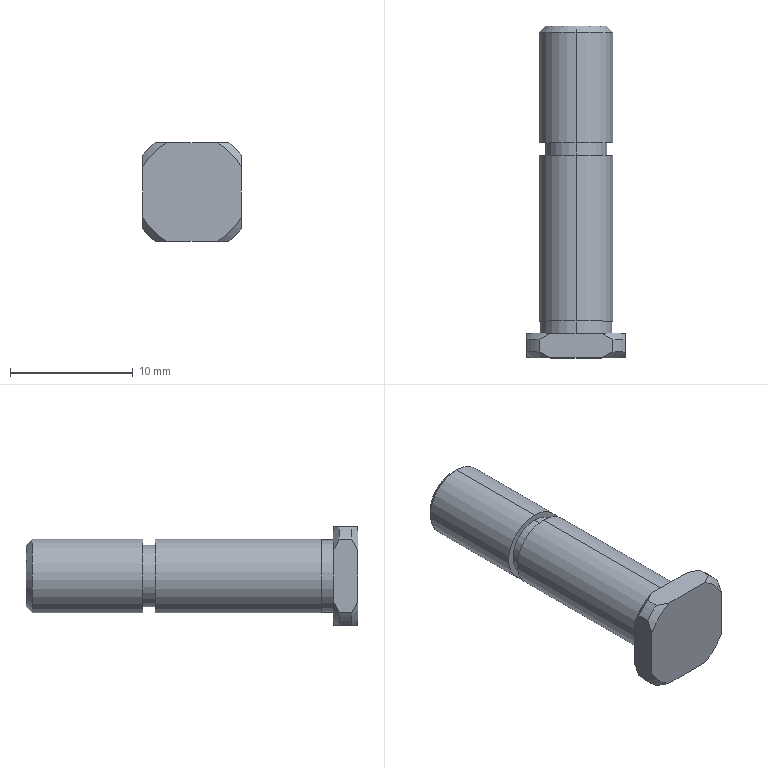Part | NX | features BREP 1 | 1 solid | 32 faces | box 8 x 27 x 8 mm | volume 818.061 mm3 | cylinder 12 | plane 10 | cone 10 | commonest cylinder face diameters 6 x4 10 x4 5 x2 5.9 x2
STEP:
#1=CARTESIAN_POINT('',(4.,0.,-2.062));
#2=VERTEX_POINT('',#1);
#3=CARTESIAN_POINT('',(4.,0.,2.062));
#4=VERTEX_POINT('',#3);
#5=CARTESIAN_POINT('',(4.,0.,-4.));
#6=DIRECTION('',(0.,0.,1.));
#7=VECTOR('',#6,1000.);
#8=LINE('',#5,#7);
#9=EDGE_CURVE('',#2,#4,#8,.T.);
#10=ORIENTED_EDGE('',*,*,#9,.F.);
#11=CARTESIAN_POINT('',(4.,0.5,-3.));
#12=VERTEX_POINT('',#11);
#13=CARTESIAN_POINT('',(4.,0.,-2.062));
#14=CARTESIAN_POINT('',(4.,0.1358,-2.358));
#15=CARTESIAN_POINT('',(4.,0.3024,-2.671));
#16=CARTESIAN_POINT('',(4.,0.5,-3.));
#17=B_SPLINE_CURVE_WITH_KNOTS('',3,(#13,#14,#15,#16),.UNSPECIFIED.,.F.,.F.,(4,4),(0.,1.),.UNSPECIFIED.);
#18=EDGE_CURVE('',#12,#2,#17,.F.);
#19=ORIENTED_EDGE('',*,*,#18,.F.);
#20=CARTESIAN_POINT('',(4.,1.5,-3.));
#21=VERTEX_POINT('',#20);
#22=CARTESIAN_POINT('',(4.,0.,-3.));
#23=DIRECTION('',(0.,-1.,0.));
#24=VECTOR('',#23,1000.);
#25=LINE('',#22,#24);
#26=EDGE_CURVE('',#21,#12,#25,.T.);
#27=ORIENTED_EDGE('',*,*,#26,.F.);
#28=CARTESIAN_POINT('',(4.,2.,-2.062));
#29=VERTEX_POINT('',#28);
#30=CARTESIAN_POINT('',(4.,1.5,-3.));
#31=CARTESIAN_POINT('',(4.,1.698,-2.671));
#32=CARTESIAN_POINT('',(4.,1.864,-2.358));
#33=CARTESIAN_POINT('',(4.,2.,-2.062));
#34=B_SPLINE_CURVE_WITH_KNOTS('',3,(#30,#31,#32,#33),.UNSPECIFIED.,.F.,.F.,(4,4),(0.,1.),.UNSPECIFIED.);
#35=EDGE_CURVE('',#29,#21,#34,.F.);
#36=ORIENTED_EDGE('',*,*,#35,.F.);
#37=CARTESIAN_POINT('',(4.,2.,2.062));
#38=VERTEX_POINT('',#37);
#39=CARTESIAN_POINT('',(4.,2.,0.));
#40=DIRECTION('',(0.,0.,-1.));
#41=VECTOR('',#40,1000.);
#42=LINE('',#39,#41);
#43=EDGE_CURVE('',#38,#29,#42,.T.);
#44=ORIENTED_EDGE('',*,*,#43,.F.);
#45=CARTESIAN_POINT('',(4.,1.5,3.));
#46=VERTEX_POINT('',#45);
#47=CARTESIAN_POINT('',(4.,2.,2.062));
#48=CARTESIAN_POINT('',(4.,1.864,2.358));
#49=CARTESIAN_POINT('',(4.,1.698,2.671));
#50=CARTESIAN_POINT('',(4.,1.5,3.));
#51=B_SPLINE_CURVE_WITH_KNOTS('',3,(#47,#48,#49,#50),.UNSPECIFIED.,.F.,.F.,(4,4),(0.,1.),.UNSPECIFIED.);
#52=EDGE_CURVE('',#46,#38,#51,.F.);
#53=ORIENTED_EDGE('',*,*,#52,.F.);
#54=CARTESIAN_POINT('',(4.,0.5,3.));
#55=VERTEX_POINT('',#54);
#56=CARTESIAN_POINT('',(4.,0.,3.));
#57=DIRECTION('',(0.,1.,0.));
#58=VECTOR('',#57,1000.);
#59=LINE('',#56,#58);
#60=EDGE_CURVE('',#55,#46,#59,.T.);
#61=ORIENTED_EDGE('',*,*,#60,.F.);
#62=CARTESIAN_POINT('',(4.,0.5,3.));
#63=CARTESIAN_POINT('',(4.,0.3024,2.671));
#64=CARTESIAN_POINT('',(4.,0.1358,2.358));
#65=CARTESIAN_POINT('',(4.,0.,2.062));
#66=B_SPLINE_CURVE_WITH_KNOTS('',3,(#62,#63,#64,#65),.UNSPECIFIED.,.F.,.F.,(4,4),(0.,1.),.UNSPECIFIED.);
#67=EDGE_CURVE('',#4,#55,#66,.F.);
#68=ORIENTED_EDGE('',*,*,#67,.F.);
#69=EDGE_LOOP('',(#10,#19,#27,#36,#44,#53,#61,#68));
#70=FACE_BOUND('',#69,.T.);
#71=CARTESIAN_POINT('',(4.,27.,-4.));
#72=DIRECTION('',(1.,0.,0.));
#73=DIRECTION('',(0.,0.,-1.));
#74=AXIS2_PLACEMENT_3D('',#71,#72,#73);
#75=PLANE('',#74);
#76=ADVANCED_FACE('',(#70),#75,.T.);
#77=CARTESIAN_POINT('',(-2.062,0.,-4.));
#78=VERTEX_POINT('',#77);
#79=CARTESIAN_POINT('',(2.062,0.,-4.));
#80=VERTEX_POINT('',#79);
#81=CARTESIAN_POINT('',(-4.,0.,-4.));
#82=DIRECTION('',(1.,0.,0.));
#83=VECTOR('',#82,1000.);
#84=LINE('',#81,#83);
#85=EDGE_CURVE('',#78,#80,#84,.T.);
#86=ORIENTED_EDGE('',*,*,#85,.F.);
#87=CARTESIAN_POINT('',(-3.,0.5,-4.));
#88=VERTEX_POINT('',#87);
#89=CARTESIAN_POINT('',(-2.062,0.,-4.));
#90=CARTESIAN_POINT('',(-2.358,0.1358,-4.));
#91=CARTESIAN_POINT('',(-2.671,0.3024,-4.));
#92=CARTESIAN_POINT('',(-3.,0.5,-4.));
#93=B_SPLINE_CURVE_WITH_KNOTS('',3,(#89,#90,#91,#92),.UNSPECIFIED.,.F.,.F.,(4,4),(0.,1.),.UNSPECIFIED.);
#94=EDGE_CURVE('',#88,#78,#93,.F.);
#95=ORIENTED_EDGE('',*,*,#94,.F.);
#96=CARTESIAN_POINT('',(-3.,1.5,-4.));
#97=VERTEX_POINT('',#96);
#98=CARTESIAN_POINT('',(-3.,0.,-4.));
#99=DIRECTION('',(0.,-1.,0.));
#100=VECTOR('',#99,1000.);
#101=LINE('',#98,#100);
#102=EDGE_CURVE('',#97,#88,#101,.T.);
#103=ORIENTED_EDGE('',*,*,#102,.F.);
#104=CARTESIAN_POINT('',(-2.062,2.,-4.));
#105=VERTEX_POINT('',#104);
#106=CARTESIAN_POINT('',(-3.,1.5,-4.));
#107=CARTESIAN_POINT('',(-2.671,1.698,-4.));
#108=CARTESIAN_POINT('',(-2.358,1.864,-4.));
#109=CARTESIAN_POINT('',(-2.062,2.,-4.));
#110=B_SPLINE_CURVE_WITH_KNOTS('',3,(#106,#107,#108,#109),.UNSPECIFIED.,.F.,.F.,(4,4),(0.,1.),.UNSPECIFIED.);
#111=EDGE_CURVE('',#105,#97,#110,.F.);
#112=ORIENTED_EDGE('',*,*,#111,.F.);
#113=CARTESIAN_POINT('',(2.062,2.,-4.));
#114=VERTEX_POINT('',#113);
#115=CARTESIAN_POINT('',(0.,2.,-4.));
#116=DIRECTION('',(-1.,0.,0.));
#117=VECTOR('',#116,1000.);
#118=LINE('',#115,#117);
#119=EDGE_CURVE('',#114,#105,#118,.T.);
#120=ORIENTED_EDGE('',*,*,#119,.F.);
#121=CARTESIAN_POINT('',(3.,1.5,-4.));
#122=VERTEX_POINT('',#121);
#123=CARTESIAN_POINT('',(2.062,2.,-4.));
#124=CARTESIAN_POINT('',(2.358,1.864,-4.));
#125=CARTESIAN_POINT('',(2.671,1.698,-4.));
#126=CARTESIAN_POINT('',(3.,1.5,-4.));
#127=B_SPLINE_CURVE_WITH_KNOTS('',3,(#123,#124,#125,#126),.UNSPECIFIED.,.F.,.F.,(4,4),(0.,1.),.UNSPECIFIED.);
#128=EDGE_CURVE('',#122,#114,#127,.F.);
#129=ORIENTED_EDGE('',*,*,#128,.F.);
#130=CARTESIAN_POINT('',(3.,0.5,-4.));
#131=VERTEX_POINT('',#130);
#132=CARTESIAN_POINT('',(3.,0.,-4.));
#133=DIRECTION('',(0.,1.,0.));
#134=VECTOR('',#133,1000.);
#135=LINE('',#132,#134);
#136=EDGE_CURVE('',#131,#122,#135,.T.);
#137=ORIENTED_EDGE('',*,*,#136,.F.);
#138=CARTESIAN_POINT('',(3.,0.5,-4.));
#139=CARTESIAN_POINT('',(2.671,0.3024,-4.));
#140=CARTESIAN_POINT('',(2.358,0.1358,-4.));
#141=CARTESIAN_POINT('',(2.062,0.,-4.));
#142=B_SPLINE_CURVE_WITH_KNOTS('',3,(#138,#139,#140,#141),.UNSPECIFIED.,.F.,.F.,(4,4),(0.,1.),.UNSPECIFIED.);
#143=EDGE_CURVE('',#80,#131,#142,.F.);
#144=ORIENTED_EDGE('',*,*,#143,.F.);
#145=EDGE_LOOP('',(#86,#95,#103,#112,#120,#129,#137,#144));
#146=FACE_BOUND('',#145,.T.);
#147=CARTESIAN_POINT('',(-4.,27.,-4.));
#148=DIRECTION('',(0.,0.,-1.));
#149=DIRECTION('',(-1.,0.,0.));
#150=AXIS2_PLACEMENT_3D('',#147,#148,#149);
#151=PLANE('',#150);
#152=ADVANCED_FACE('',(#146),#151,.T.);
#153=CARTESIAN_POINT('',(-4.,0.,2.062));
#154=VERTEX_POINT('',#153);
#155=CARTESIAN_POINT('',(-4.,0.,-2.062));
#156=VERTEX_POINT('',#155);
#157=CARTESIAN_POINT('',(-4.,0.,-4.));
#158=DIRECTION('',(0.,0.,-1.));
#159=VECTOR('',#158,1000.);
#160=LINE('',#157,#159);
#161=EDGE_CURVE('',#154,#156,#160,.T.);
#162=ORIENTED_EDGE('',*,*,#161,.F.);
#163=CARTESIAN_POINT('',(-4.,0.5,3.));
#164=VERTEX_POINT('',#163);
#165=CARTESIAN_POINT('',(-4.,0.,2.062));
#166=CARTESIAN_POINT('',(-4.,0.1358,2.358));
#167=CARTESIAN_POINT('',(-4.,0.3024,2.671));
#168=CARTESIAN_POINT('',(-4.,0.5,3.));
#169=B_SPLINE_CURVE_WITH_KNOTS('',3,(#165,#166,#167,#168),.UNSPECIFIED.,.F.,.F.,(4,4),(0.,1.),.UNSPECIFIED.);
#170=EDGE_CURVE('',#164,#154,#169,.F.);
#171=ORIENTED_EDGE('',*,*,#170,.F.);
#172=CARTESIAN_POINT('',(-4.,1.5,3.));
#173=VERTEX_POINT('',#172);
#174=CARTESIAN_POINT('',(-4.,0.,3.));
#175=DIRECTION('',(0.,-1.,0.));
#176=VECTOR('',#175,1000.);
#177=LINE('',#174,#176);
#178=EDGE_CURVE('',#173,#164,#177,.T.);
#179=ORIENTED_EDGE('',*,*,#178,.F.);
#180=CARTESIAN_POINT('',(-4.,2.,2.062));
#181=VERTEX_POINT('',#180);
#182=CARTESIAN_POINT('',(-4.,1.5,3.));
#183=CARTESIAN_POINT('',(-4.,1.698,2.671));
#184=CARTESIAN_POINT('',(-4.,1.864,2.358));
#185=CARTESIAN_POINT('',(-4.,2.,2.062));
#186=B_SPLINE_CURVE_WITH_KNOTS('',3,(#182,#183,#184,#185),.UNSPECIFIED.,.F.,.F.,(4,4),(0.,1.),.UNSPECIFIED.);
#187=EDGE_CURVE('',#181,#173,#186,.F.);
#188=ORIENTED_EDGE('',*,*,#187,.F.);
#189=CARTESIAN_POINT('',(-4.,2.,-2.062));
#190=VERTEX_POINT('',#189);
#191=CARTESIAN_POINT('',(-4.,2.,0.));
#192=DIRECTION('',(0.,0.,1.));
#193=VECTOR('',#192,1000.);
#194=LINE('',#191,#193);
#195=EDGE_CURVE('',#190,#181,#194,.T.);
#196=ORIENTED_EDGE('',*,*,#195,.F.);
#197=CARTESIAN_POINT('',(-4.,1.5,-3.));
#198=VERTEX_POINT('',#197);
#199=CARTESIAN_POINT('',(-4.,2.,-2.062));
#200=CARTESIAN_POINT('',(-4.,1.864,-2.358));
#201=CARTESIAN_POINT('',(-4.,1.698,-2.671));
#202=CARTESIAN_POINT('',(-4.,1.5,-3.));
#203=B_SPLINE_CURVE_WITH_KNOTS('',3,(#199,#200,#201,#202),.UNSPECIFIED.,.F.,.F.,(4,4),(0.,1.),.UNSPECIFIED.);
#204=EDGE_CURVE('',#198,#190,#203,.F.);
#205=ORIENTED_EDGE('',*,*,#204,.F.);
#206=CARTESIAN_POINT('',(-4.,0.5,-3.));
#207=VERTEX_POINT('',#206);
#208=CARTESIAN_POINT('',(-4.,0.,-3.));
#209=DIRECTION('',(0.,1.,0.));
#210=VECTOR('',#209,1000.);
#211=LINE('',#208,#210);
#212=EDGE_CURVE('',#207,#198,#211,.T.);
#213=ORIENTED_EDGE('',*,*,#212,.F.);
#214=CARTESIAN_POINT('',(-4.,0.5,-3.));
#215=CARTESIAN_POINT('',(-4.,0.3024,-2.671));
#216=CARTESIAN_POINT('',(-4.,0.1358,-2.358));
#217=CARTESIAN_POINT('',(-4.,0.,-2.062));
#218=B_SPLINE_CURVE_WITH_KNOTS('',3,(#214,#215,#216,#217),.UNSPECIFIED.,.F.,.F.,(4,4),(0.,1.),.UNSPECIFIED.);
#219=EDGE_CURVE('',#156,#207,#218,.F.);
#220=ORIENTED_EDGE('',*,*,#219,.F.);
#221=EDGE_LOOP('',(#162,#171,#179,#188,#196,#205,#213,#220));
#222=FACE_BOUND('',#221,.T.);
#223=CARTESIAN_POINT('',(-4.,27.,-4.));
#224=DIRECTION('',(-1.,0.,0.));
#225=DIRECTION('',(0.,0.,1.));
#226=AXIS2_PLACEMENT_3D('',#223,#224,#225);
#227=PLANE('',#226);
#228=ADVANCED_FACE('',(#222),#227,.T.);
#229=CARTESIAN_POINT('',(2.062,0.,4.));
#230=VERTEX_POINT('',#229);
#231=CARTESIAN_POINT('',(-2.062,0.,4.));
#232=VERTEX_POINT('',#231);
#233=CARTESIAN_POINT('',(-4.,0.,4.));
#234=DIRECTION('',(-1.,0.,0.));
#235=VECTOR('',#234,1000.);
#236=LINE('',#233,#235);
#237=EDGE_CURVE('',#230,#232,#236,.T.);
#238=ORIENTED_EDGE('',*,*,#237,.F.);
#239=CARTESIAN_POINT('',(3.,0.5,4.));
#240=VERTEX_POINT('',#239);
#241=CARTESIAN_POINT('',(2.062,0.,4.));
#242=CARTESIAN_POINT('',(2.358,0.1358,4.));
#243=CARTESIAN_POINT('',(2.671,0.3024,4.));
#244=CARTESIAN_POINT('',(3.,0.5,4.));
#245=B_SPLINE_CURVE_WITH_KNOTS('',3,(#241,#242,#243,#244),.UNSPECIFIED.,.F.,.F.,(4,4),(0.,1.),.UNSPECIFIED.);
#246=EDGE_CURVE('',#240,#230,#245,.F.);
#247=ORIENTED_EDGE('',*,*,#246,.F.);
#248=CARTESIAN_POINT('',(3.,1.5,4.));
#249=VERTEX_POINT('',#248);
#250=CARTESIAN_POINT('',(3.,0.,4.));
#251=DIRECTION('',(0.,-1.,0.));
#252=VECTOR('',#251,1000.);
#253=LINE('',#250,#252);
#254=EDGE_CURVE('',#249,#240,#253,.T.);
#255=ORIENTED_EDGE('',*,*,#254,.F.);
#256=CARTESIAN_POINT('',(2.062,2.,4.));
#257=VERTEX_POINT('',#256);
#258=CARTESIAN_POINT('',(3.,1.5,4.));
#259=CARTESIAN_POINT('',(2.671,1.698,4.));
#260=CARTESIAN_POINT('',(2.358,1.864,4.));
#261=CARTESIAN_POINT('',(2.062,2.,4.));
#262=B_SPLINE_CURVE_WITH_KNOTS('',3,(#258,#259,#260,#261),.UNSPECIFIED.,.F.,.F.,(4,4),(0.,1.),.UNSPECIFIED.);
#263=EDGE_CURVE('',#257,#249,#262,.F.);
#264=ORIENTED_EDGE('',*,*,#263,.F.);
#265=CARTESIAN_POINT('',(-2.062,2.,4.));
#266=VERTEX_POINT('',#265);
#267=CARTESIAN_POINT('',(0.,2.,4.));
#268=DIRECTION('',(1.,0.,0.));
#269=VECTOR('',#268,1000.);
#270=LINE('',#267,#269);
#271=EDGE_CURVE('',#266,#257,#270,.T.);
#272=ORIENTED_EDGE('',*,*,#271,.F.);
#273=CARTESIAN_POINT('',(-3.,1.5,4.));
#274=VERTEX_POINT('',#273);
#275=CARTESIAN_POINT('',(-2.062,2.,4.));
#276=CARTESIAN_POINT('',(-2.358,1.864,4.));
#277=CARTESIAN_POINT('',(-2.671,1.698,4.));
#278=CARTESIAN_POINT('',(-3.,1.5,4.));
#279=B_SPLINE_CURVE_WITH_KNOTS('',3,(#275,#276,#277,#278),.UNSPECIFIED.,.F.,.F.,(4,4),(0.,1.),.UNSPECIFIED.);
#280=EDGE_CURVE('',#274,#266,#279,.F.);
#281=ORIENTED_EDGE('',*,*,#280,.F.);
#282=CARTESIAN_POINT('',(-3.,0.5,4.));
#283=VERTEX_POINT('',#282);
#284=CARTESIAN_POINT('',(-3.,0.,4.));
#285=DIRECTION('',(0.,1.,0.));
#286=VECTOR('',#285,1000.);
#287=LINE('',#284,#286);
#288=EDGE_CURVE('',#283,#274,#287,.T.);
#289=ORIENTED_EDGE('',*,*,#288,.F.);
#290=CARTESIAN_POINT('',(-3.,0.5,4.));
#291=CARTESIAN_POINT('',(-2.671,0.3024,4.));
#292=CARTESIAN_POINT('',(-2.358,0.1358,4.));
#293=CARTESIAN_POINT('',(-2.062,0.,4.));
#294=B_SPLINE_CURVE_WITH_KNOTS('',3,(#290,#291,#292,#293),.UNSPECIFIED.,.F.,.F.,(4,4),(0.,1.),.UNSPECIFIED.);
#295=EDGE_CURVE('',#232,#283,#294,.F.);
#296=ORIENTED_EDGE('',*,*,#295,.F.);
#297=EDGE_LOOP('',(#238,#247,#255,#264,#272,#281,#289,#296));
#298=FACE_BOUND('',#297,.T.);
#299=CARTESIAN_POINT('',(-4.,27.,4.));
#300=DIRECTION('',(0.,0.,1.));
#301=DIRECTION('',(1.,0.,0.));
#302=AXIS2_PLACEMENT_3D('',#299,#300,#301);
#303=PLANE('',#302);
#304=ADVANCED_FACE('',(#298),#303,.T.);
#305=CARTESIAN_POINT('',(0.,27.,2.5));
#306=VERTEX_POINT('',#305);
#307=CARTESIAN_POINT('',(0.,26.5,3.));
#308=VERTEX_POINT('',#307);
#309=CARTESIAN_POINT('',(0.,27.,2.5));
#310=DIRECTION('',(0.,-0.7071,0.7071));
#311=VECTOR('',#310,1000.);
#312=LINE('',#309,#311);
#313=EDGE_CURVE('',#306,#308,#312,.T.);
#314=ORIENTED_EDGE('',*,*,#313,.F.);
#315=CARTESIAN_POINT('',(0.,27.,-2.5));
#316=VERTEX_POINT('',#315);
#317=CARTESIAN_POINT('',(0.,27.,0.));
#318=DIRECTION('',(0.,1.,0.));
#319=DIRECTION('',(0.,0.,1.));
#320=AXIS2_PLACEMENT_3D('',#317,#318,#319);
#321=CIRCLE('',#320,2.5);
#322=EDGE_CURVE('',#316,#306,#321,.T.);
#323=ORIENTED_EDGE('',*,*,#322,.F.);
#324=CARTESIAN_POINT('',(0.,26.5,-3.));
#325=VERTEX_POINT('',#324);
#326=CARTESIAN_POINT('',(0.,27.,-2.5));
#327=DIRECTION('',(0.,-0.7071,-0.7071));
#328=VECTOR('',#327,1000.);
#329=LINE('',#326,#328);
#330=EDGE_CURVE('',#316,#325,#329,.T.);
#331=ORIENTED_EDGE('',*,*,#330,.T.);
#332=CARTESIAN_POINT('',(0.,26.5,0.));
#333=DIRECTION('',(0.,-1.,0.));
#334=DIRECTION('',(0.,0.,1.));
#335=AXIS2_PLACEMENT_3D('',#332,#333,#334);
#336=CIRCLE('',#335,3.);
#337=EDGE_CURVE('',#308,#325,#336,.T.);
#338=ORIENTED_EDGE('',*,*,#337,.F.);
#339=EDGE_LOOP('',(#314,#323,#331,#338));
#340=FACE_BOUND('',#339,.T.);
#341=CARTESIAN_POINT('',(0.,27.,0.));
#342=DIRECTION('',(0.,-1.,0.));
#343=DIRECTION('',(0.,0.,-1.));
#344=AXIS2_PLACEMENT_3D('',#341,#342,#343);
#345=CONICAL_SURFACE('',#344,2.5,0.7854);
#346=ADVANCED_FACE('',(#340),#345,.T.);
#347=CARTESIAN_POINT('',(0.,3.,2.95));
#348=VERTEX_POINT('',#347);
#349=CARTESIAN_POINT('',(0.,2.,2.95));
#350=VERTEX_POINT('',#349);
#351=CARTESIAN_POINT('',(0.,3.,2.95));
#352=DIRECTION('',(0.,-1.,0.));
#353=VECTOR('',#352,1000.);
#354=LINE('',#351,#353);
#355=EDGE_CURVE('',#348,#350,#354,.T.);
#356=ORIENTED_EDGE('',*,*,#355,.F.);
#357=CARTESIAN_POINT('',(0.,3.,-2.95));
#358=VERTEX_POINT('',#357);
#359=CARTESIAN_POINT('',(0.,3.,0.));
#360=DIRECTION('',(0.,1.,0.));
#361=DIRECTION('',(0.,0.,1.));
#362=AXIS2_PLACEMENT_3D('',#359,#360,#361);
#363=CIRCLE('',#362,2.95);
#364=EDGE_CURVE('',#358,#348,#363,.T.);
#365=ORIENTED_EDGE('',*,*,#364,.F.);
#366=CARTESIAN_POINT('',(0.,2.,-2.95));
#367=VERTEX_POINT('',#366);
#368=CARTESIAN_POINT('',(0.,3.,-2.95));
#369=DIRECTION('',(0.,-1.,0.));
#370=VECTOR('',#369,1000.);
#371=LINE('',#368,#370);
#372=EDGE_CURVE('',#358,#367,#371,.T.);
#373=ORIENTED_EDGE('',*,*,#372,.T.);
#374=CARTESIAN_POINT('',(0.,2.,0.));
#375=DIRECTION('',(0.,1.,0.));
#376=DIRECTION('',(0.,0.,1.));
#377=AXIS2_PLACEMENT_3D('',#374,#375,#376);
#378=CIRCLE('',#377,2.95);
#379=EDGE_CURVE('',#367,#350,#378,.T.);
#380=ORIENTED_EDGE('',*,*,#379,.T.);
#381=EDGE_LOOP('',(#356,#365,#373,#380));
#382=FACE_BOUND('',#381,.T.);
#383=CARTESIAN_POINT('',(0.,3.,0.));
#384=DIRECTION('',(0.,-1.,0.));
#385=DIRECTION('',(0.,0.,-1.));
#386=AXIS2_PLACEMENT_3D('',#383,#384,#385);
#387=CYLINDRICAL_SURFACE('',#386,2.95);
#388=ADVANCED_FACE('',(#382),#387,.T.);
#389=ORIENTED_EDGE('',*,*,#364,.T.);
#390=CARTESIAN_POINT('',(0.,3.,0.));
#391=DIRECTION('',(0.,1.,0.));
#392=DIRECTION('',(0.,0.,1.));
#393=AXIS2_PLACEMENT_3D('',#390,#391,#392);
#394=CIRCLE('',#393,2.95);
#395=EDGE_CURVE('',#348,#358,#394,.T.);
#396=ORIENTED_EDGE('',*,*,#395,.T.);
#397=EDGE_LOOP('',(#389,#396));
#398=FACE_BOUND('',#397,.T.);
#399=CARTESIAN_POINT('',(0.,3.,3.));
#400=VERTEX_POINT('',#399);
#401=CARTESIAN_POINT('',(0.,3.,-3.));
#402=VERTEX_POINT('',#401);
#403=CARTESIAN_POINT('',(0.,3.,0.));
#404=DIRECTION('',(0.,-1.,0.));
#405=DIRECTION('',(0.,0.,1.));
#406=AXIS2_PLACEMENT_3D('',#403,#404,#405);
#407=CIRCLE('',#406,3.);
#408=EDGE_CURVE('',#400,#402,#407,.T.);
#409=ORIENTED_EDGE('',*,*,#408,.T.);
#410=CARTESIAN_POINT('',(0.,3.,0.));
#411=DIRECTION('',(0.,-1.,0.));
#412=DIRECTION('',(0.,0.,1.));
#413=AXIS2_PLACEMENT_3D('',#410,#411,#412);
#414=CIRCLE('',#413,3.);
#415=EDGE_CURVE('',#402,#400,#414,.T.);
#416=ORIENTED_EDGE('',*,*,#415,.T.);
#417=EDGE_LOOP('',(#409,#416));
#418=FACE_BOUND('',#417,.T.);
#419=CARTESIAN_POINT('',(0.,3.,0.));
#420=DIRECTION('',(0.,1.,0.));
#421=DIRECTION('',(0.,0.,1.));
#422=AXIS2_PLACEMENT_3D('',#419,#420,#421);
#423=PLANE('',#422);
#424=ADVANCED_FACE('',(#398,#418),#423,.F.);
#425=CARTESIAN_POINT('',(0.,17.5,3.));
#426=VERTEX_POINT('',#425);
#427=CARTESIAN_POINT('',(0.,17.5,-3.));
#428=VERTEX_POINT('',#427);
#429=CARTESIAN_POINT('',(0.,17.5,0.));
#430=DIRECTION('',(0.,1.,0.));
#431=DIRECTION('',(0.,0.,1.));
#432=AXIS2_PLACEMENT_3D('',#429,#430,#431);
#433=CIRCLE('',#432,3.);
#434=EDGE_CURVE('',#426,#428,#433,.T.);
#435=ORIENTED_EDGE('',*,*,#434,.F.);
#436=CARTESIAN_POINT('',(0.,17.5,0.));
#437=DIRECTION('',(0.,1.,0.));
#438=DIRECTION('',(0.,0.,1.));
#439=AXIS2_PLACEMENT_3D('',#436,#437,#438);
#440=CIRCLE('',#439,3.);
#441=EDGE_CURVE('',#428,#426,#440,.T.);
#442=ORIENTED_EDGE('',*,*,#441,.F.);
#443=EDGE_LOOP('',(#435,#442));
#444=FACE_BOUND('',#443,.T.);
#445=CARTESIAN_POINT('',(0.,17.5,2.5));
#446=VERTEX_POINT('',#445);
#447=CARTESIAN_POINT('',(0.,17.5,-2.5));
#448=VERTEX_POINT('',#447);
#449=CARTESIAN_POINT('',(0.,17.5,0.));
#450=DIRECTION('',(0.,1.,0.));
#451=DIRECTION('',(0.,0.,1.));
#452=AXIS2_PLACEMENT_3D('',#449,#450,#451);
#453=CIRCLE('',#452,2.5);
#454=EDGE_CURVE('',#446,#448,#453,.T.);
#455=ORIENTED_EDGE('',*,*,#454,.T.);
#456=CARTESIAN_POINT('',(0.,17.5,0.));
#457=DIRECTION('',(0.,1.,0.));
#458=DIRECTION('',(0.,0.,1.));
#459=AXIS2_PLACEMENT_3D('',#456,#457,#458);
#460=CIRCLE('',#459,2.5);
#461=EDGE_CURVE('',#448,#446,#460,.T.);
#462=ORIENTED_EDGE('',*,*,#461,.T.);
#463=EDGE_LOOP('',(#455,#462));
#464=FACE_BOUND('',#463,.T.);
#465=CARTESIAN_POINT('',(0.,17.5,0.));
#466=DIRECTION('',(0.,-1.,0.));
#467=DIRECTION('',(0.,0.,-1.));
#468=AXIS2_PLACEMENT_3D('',#465,#466,#467);
#469=PLANE('',#468);
#470=ADVANCED_FACE('',(#444,#464),#469,.T.);
#471=CARTESIAN_POINT('',(0.,0.,-3.));
#472=DIRECTION('',(0.,1.,0.));
#473=VECTOR('',#472,1000.);
#474=LINE('',#471,#473);
#475=EDGE_CURVE('',#325,#428,#474,.F.);
#476=ORIENTED_EDGE('',*,*,#475,.T.);
#477=ORIENTED_EDGE('',*,*,#441,.T.);
#478=CARTESIAN_POINT('',(0.,0.,3.));
#479=DIRECTION('',(0.,1.,0.));
#480=VECTOR('',#479,1000.);
#481=LINE('',#478,#480);
#482=EDGE_CURVE('',#308,#426,#481,.F.);
#483=ORIENTED_EDGE('',*,*,#482,.F.);
#484=ORIENTED_EDGE('',*,*,#337,.T.);
#485=EDGE_LOOP('',(#476,#477,#483,#484));
#486=FACE_BOUND('',#485,.T.);
#487=CARTESIAN_POINT('',(0.,0.,0.));
#488=DIRECTION('',(0.,1.,0.));
#489=DIRECTION('',(0.,0.,1.));
#490=AXIS2_PLACEMENT_3D('',#487,#488,#489);
#491=CYLINDRICAL_SURFACE('',#490,3.);
#492=ADVANCED_FACE('',(#486),#491,.T.);
#493=ORIENTED_EDGE('',*,*,#322,.T.);
#494=CARTESIAN_POINT('',(0.,27.,0.));
#495=DIRECTION('',(0.,1.,0.));
#496=DIRECTION('',(0.,0.,1.));
#497=AXIS2_PLACEMENT_3D('',#494,#495,#496);
#498=CIRCLE('',#497,2.5);
#499=EDGE_CURVE('',#306,#316,#498,.T.);
#500=ORIENTED_EDGE('',*,*,#499,.T.);
#501=EDGE_LOOP('',(#493,#500));
#502=FACE_BOUND('',#501,.T.);
#503=CARTESIAN_POINT('',(0.,27.,0.));
#504=DIRECTION('',(0.,1.,0.));
#505=DIRECTION('',(0.,0.,1.));
#506=AXIS2_PLACEMENT_3D('',#503,#504,#505);
#507=PLANE('',#506);
#508=ADVANCED_FACE('',(#502),#507,.T.);
#509=CARTESIAN_POINT('',(0.,16.5,-3.));
#510=VERTEX_POINT('',#509);
#511=CARTESIAN_POINT('',(0.,0.,-3.));
#512=DIRECTION('',(0.,1.,0.));
#513=VECTOR('',#512,1000.);
#514=LINE('',#511,#513);
#515=EDGE_CURVE('',#510,#402,#514,.F.);
#516=ORIENTED_EDGE('',*,*,#515,.T.);
#517=ORIENTED_EDGE('',*,*,#408,.F.);
#518=CARTESIAN_POINT('',(0.,16.5,3.));
#519=VERTEX_POINT('',#518);
#520=CARTESIAN_POINT('',(0.,0.,3.));
#521=DIRECTION('',(0.,1.,0.));
#522=VECTOR('',#521,1000.);
#523=LINE('',#520,#522);
#524=EDGE_CURVE('',#519,#400,#523,.F.);
#525=ORIENTED_EDGE('',*,*,#524,.F.);
#526=CARTESIAN_POINT('',(0.,16.5,0.));
#527=DIRECTION('',(0.,1.,0.));
#528=DIRECTION('',(0.,0.,1.));
#529=AXIS2_PLACEMENT_3D('',#526,#527,#528);
#530=CIRCLE('',#529,3.);
#531=EDGE_CURVE('',#510,#519,#530,.T.);
#532=ORIENTED_EDGE('',*,*,#531,.F.);
#533=EDGE_LOOP('',(#516,#517,#525,#532));
#534=FACE_BOUND('',#533,.T.);
#535=CARTESIAN_POINT('',(0.,0.,0.));
#536=DIRECTION('',(0.,1.,0.));
#537=DIRECTION('',(0.,0.,1.));
#538=AXIS2_PLACEMENT_3D('',#535,#536,#537);
#539=CYLINDRICAL_SURFACE('',#538,3.);
#540=ADVANCED_FACE('',(#534),#539,.T.);
#541=CARTESIAN_POINT('',(0.,16.5,0.));
#542=DIRECTION('',(0.,1.,0.));
#543=DIRECTION('',(0.,0.,1.));
#544=AXIS2_PLACEMENT_3D('',#541,#542,#543);
#545=CIRCLE('',#544,3.);
#546=EDGE_CURVE('',#519,#510,#545,.T.);
#547=ORIENTED_EDGE('',*,*,#546,.T.);
#548=ORIENTED_EDGE('',*,*,#531,.T.);
#549=EDGE_LOOP('',(#547,#548));
#550=FACE_BOUND('',#549,.T.);
#551=CARTESIAN_POINT('',(0.,16.5,2.5));
#552=VERTEX_POINT('',#551);
#553=CARTESIAN_POINT('',(0.,16.5,-2.5));
#554=VERTEX_POINT('',#553);
#555=CARTESIAN_POINT('',(0.,16.5,0.));
#556=DIRECTION('',(0.,1.,0.));
#557=DIRECTION('',(0.,0.,1.));
#558=AXIS2_PLACEMENT_3D('',#555,#556,#557);
#559=CIRCLE('',#558,2.5);
#560=EDGE_CURVE('',#552,#554,#559,.T.);
#561=ORIENTED_EDGE('',*,*,#560,.F.);
#562=CARTESIAN_POINT('',(0.,16.5,0.));
#563=DIRECTION('',(0.,1.,0.));
#564=DIRECTION('',(0.,0.,1.));
#565=AXIS2_PLACEMENT_3D('',#562,#563,#564);
#566=CIRCLE('',#565,2.5);
#567=EDGE_CURVE('',#554,#552,#566,.T.);
#568=ORIENTED_EDGE('',*,*,#567,.F.);
#569=EDGE_LOOP('',(#561,#568));
#570=FACE_BOUND('',#569,.T.);
#571=CARTESIAN_POINT('',(0.,16.5,0.));
#572=DIRECTION('',(0.,-1.,0.));
#573=DIRECTION('',(0.,0.,-1.));
#574=AXIS2_PLACEMENT_3D('',#571,#572,#573);
#575=PLANE('',#574);
#576=ADVANCED_FACE('',(#550,#570),#575,.F.);
#577=CARTESIAN_POINT('',(0.,0.,-2.5));
#578=DIRECTION('',(0.,1.,0.));
#579=VECTOR('',#578,1000.);
#580=LINE('',#577,#579);
#581=EDGE_CURVE('',#448,#554,#580,.F.);
#582=ORIENTED_EDGE('',*,*,#581,.T.);
#583=ORIENTED_EDGE('',*,*,#567,.T.);
#584=CARTESIAN_POINT('',(0.,0.,2.5));
#585=DIRECTION('',(0.,1.,0.));
#586=VECTOR('',#585,1000.);
#587=LINE('',#584,#586);
#588=EDGE_CURVE('',#446,#552,#587,.F.);
#589=ORIENTED_EDGE('',*,*,#588,.F.);
#590=ORIENTED_EDGE('',*,*,#461,.F.);
#591=EDGE_LOOP('',(#582,#583,#589,#590));
#592=FACE_BOUND('',#591,.T.);
#593=CARTESIAN_POINT('',(0.,0.,0.));
#594=DIRECTION('',(0.,1.,0.));
#595=DIRECTION('',(0.,0.,1.));
#596=AXIS2_PLACEMENT_3D('',#593,#594,#595);
#597=CYLINDRICAL_SURFACE('',#596,2.5);
#598=ADVANCED_FACE('',(#592),#597,.T.);
#599=CARTESIAN_POINT('',(0.,2.,0.));
#600=DIRECTION('',(0.,1.,0.));
#601=DIRECTION('',(0.,0.,1.));
#602=AXIS2_PLACEMENT_3D('',#599,#600,#601);
#603=CIRCLE('',#602,4.5);
#604=EDGE_CURVE('',#181,#266,#603,.T.);
#605=ORIENTED_EDGE('',*,*,#604,.F.);
#606=ORIENTED_EDGE('',*,*,#187,.T.);
#607=CARTESIAN_POINT('',(0.,1.5,0.));
#608=DIRECTION('',(0.,-1.,0.));
#609=DIRECTION('',(0.,0.,1.));
#610=AXIS2_PLACEMENT_3D('',#607,#608,#609);
#611=CIRCLE('',#610,5.);
#612=EDGE_CURVE('',#274,#173,#611,.T.);
#613=ORIENTED_EDGE('',*,*,#612,.F.);
#614=ORIENTED_EDGE('',*,*,#280,.T.);
#615=EDGE_LOOP('',(#605,#606,#613,#614));
#616=FACE_BOUND('',#615,.T.);
#617=CARTESIAN_POINT('',(0.,2.,0.));
#618=DIRECTION('',(0.,-1.,0.));
#619=DIRECTION('',(0.,0.,-1.));
#620=AXIS2_PLACEMENT_3D('',#617,#618,#619);
#621=CONICAL_SURFACE('',#620,4.5,0.7854);
#622=ADVANCED_FACE('',(#616),#621,.T.);
#623=CARTESIAN_POINT('',(0.,2.,0.));
#624=DIRECTION('',(0.,1.,0.));
#625=DIRECTION('',(0.,0.,1.));
#626=AXIS2_PLACEMENT_3D('',#623,#624,#625);
#627=CIRCLE('',#626,4.5);
#628=EDGE_CURVE('',#105,#190,#627,.T.);
#629=ORIENTED_EDGE('',*,*,#628,.F.);
#630=ORIENTED_EDGE('',*,*,#111,.T.);
#631=CARTESIAN_POINT('',(0.,1.5,0.));
#632=DIRECTION('',(0.,-1.,0.));
#633=DIRECTION('',(0.,0.,1.));
#634=AXIS2_PLACEMENT_3D('',#631,#632,#633);
#635=CIRCLE('',#634,5.);
#636=EDGE_CURVE('',#198,#97,#635,.T.);
#637=ORIENTED_EDGE('',*,*,#636,.F.);
#638=ORIENTED_EDGE('',*,*,#204,.T.);
#639=EDGE_LOOP('',(#629,#630,#637,#638));
#640=FACE_BOUND('',#639,.T.);
#641=CARTESIAN_POINT('',(0.,2.,0.));
#642=DIRECTION('',(0.,-1.,0.));
#643=DIRECTION('',(0.,0.,-1.));
#644=AXIS2_PLACEMENT_3D('',#641,#642,#643);
#645=CONICAL_SURFACE('',#644,4.5,0.7854);
#646=ADVANCED_FACE('',(#640),#645,.T.);
#647=CARTESIAN_POINT('',(0.,2.,0.));
#648=DIRECTION('',(0.,1.,0.));
#649=DIRECTION('',(0.,0.,1.));
#650=AXIS2_PLACEMENT_3D('',#647,#648,#649);
#651=CIRCLE('',#650,4.5);
#652=EDGE_CURVE('',#29,#114,#651,.T.);
#653=ORIENTED_EDGE('',*,*,#652,.F.);
#654=ORIENTED_EDGE('',*,*,#35,.T.);
#655=CARTESIAN_POINT('',(0.,1.5,0.));
#656=DIRECTION('',(0.,-1.,0.));
#657=DIRECTION('',(0.,0.,1.));
#658=AXIS2_PLACEMENT_3D('',#655,#656,#657);
#659=CIRCLE('',#658,5.);
#660=EDGE_CURVE('',#122,#21,#659,.T.);
#661=ORIENTED_EDGE('',*,*,#660,.F.);
#662=ORIENTED_EDGE('',*,*,#128,.T.);
#663=EDGE_LOOP('',(#653,#654,#661,#662));
#664=FACE_BOUND('',#663,.T.);
#665=CARTESIAN_POINT('',(0.,2.,0.));
#666=DIRECTION('',(0.,-1.,0.));
#667=DIRECTION('',(0.,0.,-1.));
#668=AXIS2_PLACEMENT_3D('',#665,#666,#667);
#669=CONICAL_SURFACE('',#668,4.5,0.7854);
#670=ADVANCED_FACE('',(#664),#669,.T.);
#671=CARTESIAN_POINT('',(0.,1.5,0.));
#672=DIRECTION('',(0.,-1.,0.));
#673=DIRECTION('',(0.,0.,1.));
#674=AXIS2_PLACEMENT_3D('',#671,#672,#673);
#675=CIRCLE('',#674,5.);
#676=EDGE_CURVE('',#46,#249,#675,.T.);
#677=ORIENTED_EDGE('',*,*,#676,.F.);
#678=ORIENTED_EDGE('',*,*,#52,.T.);
#679=CARTESIAN_POINT('',(0.,2.,0.));
#680=DIRECTION('',(0.,1.,0.));
#681=DIRECTION('',(0.,0.,1.));
#682=AXIS2_PLACEMENT_3D('',#679,#680,#681);
#683=CIRCLE('',#682,4.5);
#684=EDGE_CURVE('',#257,#38,#683,.T.);
#685=ORIENTED_EDGE('',*,*,#684,.F.);
#686=ORIENTED_EDGE('',*,*,#263,.T.);
#687=EDGE_LOOP('',(#677,#678,#685,#686));
#688=FACE_BOUND('',#687,.T.);
#689=CARTESIAN_POINT('',(0.,2.,0.));
#690=DIRECTION('',(0.,-1.,0.));
#691=DIRECTION('',(0.,0.,-1.));
#692=AXIS2_PLACEMENT_3D('',#689,#690,#691);
#693=CONICAL_SURFACE('',#692,4.5,0.7854);
#694=ADVANCED_FACE('',(#688),#693,.T.);
#695=CARTESIAN_POINT('',(0.,0.5,0.));
#696=DIRECTION('',(0.,1.,0.));
#697=DIRECTION('',(0.,0.,-1.));
#698=AXIS2_PLACEMENT_3D('',#695,#696,#697);
#699=CIRCLE('',#698,5.);
#700=EDGE_CURVE('',#164,#283,#699,.T.);
#701=ORIENTED_EDGE('',*,*,#700,.F.);
#702=ORIENTED_EDGE('',*,*,#170,.T.);
#703=CARTESIAN_POINT('',(0.,0.,0.));
#704=DIRECTION('',(0.,-1.,0.));
#705=DIRECTION('',(0.,0.,-1.));
#706=AXIS2_PLACEMENT_3D('',#703,#704,#705);
#707=CIRCLE('',#706,4.5);
#708=EDGE_CURVE('',#232,#154,#707,.T.);
#709=ORIENTED_EDGE('',*,*,#708,.F.);
#710=ORIENTED_EDGE('',*,*,#295,.T.);
#711=EDGE_LOOP('',(#701,#702,#709,#710));
#712=FACE_BOUND('',#711,.T.);
#713=CARTESIAN_POINT('',(0.,0.5,0.));
#714=DIRECTION('',(0.,1.,0.));
#715=DIRECTION('',(0.,0.,1.));
#716=AXIS2_PLACEMENT_3D('',#713,#714,#715);
#717=CONICAL_SURFACE('',#716,5.,0.7854);
#718=ADVANCED_FACE('',(#712),#717,.T.);
#719=CARTESIAN_POINT('',(0.,0.5,0.));
#720=DIRECTION('',(0.,1.,0.));
#721=DIRECTION('',(0.,0.,-1.));
#722=AXIS2_PLACEMENT_3D('',#719,#720,#721);
#723=CIRCLE('',#722,5.);
#724=EDGE_CURVE('',#88,#207,#723,.T.);
#725=ORIENTED_EDGE('',*,*,#724,.F.);
#726=ORIENTED_EDGE('',*,*,#94,.T.);
#727=CARTESIAN_POINT('',(0.,0.,0.));
#728=DIRECTION('',(0.,-1.,0.));
#729=DIRECTION('',(0.,0.,-1.));
#730=AXIS2_PLACEMENT_3D('',#727,#728,#729);
#731=CIRCLE('',#730,4.5);
#732=EDGE_CURVE('',#156,#78,#731,.T.);
#733=ORIENTED_EDGE('',*,*,#732,.F.);
#734=ORIENTED_EDGE('',*,*,#219,.T.);
#735=EDGE_LOOP('',(#725,#726,#733,#734));
#736=FACE_BOUND('',#735,.T.);
#737=CARTESIAN_POINT('',(0.,0.5,0.));
#738=DIRECTION('',(0.,1.,0.));
#739=DIRECTION('',(0.,0.,1.));
#740=AXIS2_PLACEMENT_3D('',#737,#738,#739);
#741=CONICAL_SURFACE('',#740,5.,0.7854);
#742=ADVANCED_FACE('',(#736),#741,.T.);
#743=CARTESIAN_POINT('',(0.,0.,0.));
#744=DIRECTION('',(0.,-1.,0.));
#745=DIRECTION('',(0.,0.,-1.));
#746=AXIS2_PLACEMENT_3D('',#743,#744,#745);
#747=CIRCLE('',#746,4.5);
#748=EDGE_CURVE('',#4,#230,#747,.T.);
#749=ORIENTED_EDGE('',*,*,#748,.F.);
#750=ORIENTED_EDGE('',*,*,#67,.T.);
#751=CARTESIAN_POINT('',(0.,0.5,0.));
#752=DIRECTION('',(0.,1.,0.));
#753=DIRECTION('',(0.,0.,-1.));
#754=AXIS2_PLACEMENT_3D('',#751,#752,#753);
#755=CIRCLE('',#754,5.);
#756=EDGE_CURVE('',#240,#55,#755,.T.);
#757=ORIENTED_EDGE('',*,*,#756,.F.);
#758=ORIENTED_EDGE('',*,*,#246,.T.);
#759=EDGE_LOOP('',(#749,#750,#757,#758));
#760=FACE_BOUND('',#759,.T.);
#761=CARTESIAN_POINT('',(0.,0.5,0.));
#762=DIRECTION('',(0.,1.,0.));
#763=DIRECTION('',(0.,0.,1.));
#764=AXIS2_PLACEMENT_3D('',#761,#762,#763);
#765=CONICAL_SURFACE('',#764,5.,0.7854);
#766=ADVANCED_FACE('',(#760),#765,.T.);
#767=CARTESIAN_POINT('',(0.,0.5,0.));
#768=DIRECTION('',(0.,1.,0.));
#769=DIRECTION('',(0.,0.,-1.));
#770=AXIS2_PLACEMENT_3D('',#767,#768,#769);
#771=CIRCLE('',#770,5.);
#772=EDGE_CURVE('',#12,#131,#771,.T.);
#773=ORIENTED_EDGE('',*,*,#772,.F.);
#774=ORIENTED_EDGE('',*,*,#18,.T.);
#775=CARTESIAN_POINT('',(0.,0.,0.));
#776=DIRECTION('',(0.,-1.,0.));
#777=DIRECTION('',(0.,0.,-1.));
#778=AXIS2_PLACEMENT_3D('',#775,#776,#777);
#779=CIRCLE('',#778,4.5);
#780=EDGE_CURVE('',#80,#2,#779,.T.);
#781=ORIENTED_EDGE('',*,*,#780,.F.);
#782=ORIENTED_EDGE('',*,*,#143,.T.);
#783=EDGE_LOOP('',(#773,#774,#781,#782));
#784=FACE_BOUND('',#783,.T.);
#785=CARTESIAN_POINT('',(0.,0.5,0.));
#786=DIRECTION('',(0.,1.,0.));
#787=DIRECTION('',(0.,0.,1.));
#788=AXIS2_PLACEMENT_3D('',#785,#786,#787);
#789=CONICAL_SURFACE('',#788,5.,0.7854);
#790=ADVANCED_FACE('',(#784),#789,.T.);
#791=ORIENTED_EDGE('',*,*,#684,.T.);
#792=ORIENTED_EDGE('',*,*,#43,.T.);
#793=ORIENTED_EDGE('',*,*,#652,.T.);
#794=ORIENTED_EDGE('',*,*,#119,.T.);
#795=ORIENTED_EDGE('',*,*,#628,.T.);
#796=ORIENTED_EDGE('',*,*,#195,.T.);
#797=ORIENTED_EDGE('',*,*,#604,.T.);
#798=ORIENTED_EDGE('',*,*,#271,.T.);
#799=EDGE_LOOP('',(#791,#792,#793,#794,#795,#796,#797,#798));
#800=FACE_BOUND('',#799,.T.);
#801=ORIENTED_EDGE('',*,*,#379,.F.);
#802=CARTESIAN_POINT('',(0.,2.,0.));
#803=DIRECTION('',(0.,1.,0.));
#804=DIRECTION('',(0.,0.,1.));
#805=AXIS2_PLACEMENT_3D('',#802,#803,#804);
#806=CIRCLE('',#805,2.95);
#807=EDGE_CURVE('',#350,#367,#806,.T.);
#808=ORIENTED_EDGE('',*,*,#807,.F.);
#809=EDGE_LOOP('',(#801,#808));
#810=FACE_BOUND('',#809,.T.);
#811=CARTESIAN_POINT('',(0.,2.,0.));
#812=DIRECTION('',(0.,1.,0.));
#813=DIRECTION('',(0.,0.,1.));
#814=AXIS2_PLACEMENT_3D('',#811,#812,#813);
#815=PLANE('',#814);
#816=ADVANCED_FACE('',(#800,#810),#815,.T.);
#817=ORIENTED_EDGE('',*,*,#612,.T.);
#818=ORIENTED_EDGE('',*,*,#178,.T.);
#819=ORIENTED_EDGE('',*,*,#700,.T.);
#820=ORIENTED_EDGE('',*,*,#288,.T.);
#821=EDGE_LOOP('',(#817,#818,#819,#820));
#822=FACE_BOUND('',#821,.T.);
#823=CARTESIAN_POINT('',(0.,0.,0.));
#824=DIRECTION('',(0.,1.,0.));
#825=DIRECTION('',(0.,0.,1.));
#826=AXIS2_PLACEMENT_3D('',#823,#824,#825);
#827=CYLINDRICAL_SURFACE('',#826,5.);
#828=ADVANCED_FACE('',(#822),#827,.T.);
#829=ORIENTED_EDGE('',*,*,#636,.T.);
#830=ORIENTED_EDGE('',*,*,#102,.T.);
#831=ORIENTED_EDGE('',*,*,#724,.T.);
#832=ORIENTED_EDGE('',*,*,#212,.T.);
#833=EDGE_LOOP('',(#829,#830,#831,#832));
#834=FACE_BOUND('',#833,.T.);
#835=CARTESIAN_POINT('',(0.,0.,0.));
#836=DIRECTION('',(0.,1.,0.));
#837=DIRECTION('',(0.,0.,1.));
#838=AXIS2_PLACEMENT_3D('',#835,#836,#837);
#839=CYLINDRICAL_SURFACE('',#838,5.);
#840=ADVANCED_FACE('',(#834),#839,.T.);
#841=ORIENTED_EDGE('',*,*,#756,.T.);
#842=ORIENTED_EDGE('',*,*,#60,.T.);
#843=ORIENTED_EDGE('',*,*,#676,.T.);
#844=ORIENTED_EDGE('',*,*,#254,.T.);
#845=EDGE_LOOP('',(#841,#842,#843,#844));
#846=FACE_BOUND('',#845,.T.);
#847=CARTESIAN_POINT('',(0.,0.,0.));
#848=DIRECTION('',(0.,1.,0.));
#849=DIRECTION('',(0.,0.,1.));
#850=AXIS2_PLACEMENT_3D('',#847,#848,#849);
#851=CYLINDRICAL_SURFACE('',#850,5.);
#852=ADVANCED_FACE('',(#846),#851,.T.);
#853=ORIENTED_EDGE('',*,*,#660,.T.);
#854=ORIENTED_EDGE('',*,*,#26,.T.);
#855=ORIENTED_EDGE('',*,*,#772,.T.);
#856=ORIENTED_EDGE('',*,*,#136,.T.);
#857=EDGE_LOOP('',(#853,#854,#855,#856));
#858=FACE_BOUND('',#857,.T.);
#859=CARTESIAN_POINT('',(0.,0.,0.));
#860=DIRECTION('',(0.,1.,0.));
#861=DIRECTION('',(0.,0.,1.));
#862=AXIS2_PLACEMENT_3D('',#859,#860,#861);
#863=CYLINDRICAL_SURFACE('',#862,5.);
#864=ADVANCED_FACE('',(#858),#863,.T.);
#865=ORIENTED_EDGE('',*,*,#780,.T.);
#866=ORIENTED_EDGE('',*,*,#9,.T.);
#867=ORIENTED_EDGE('',*,*,#748,.T.);
#868=ORIENTED_EDGE('',*,*,#237,.T.);
#869=ORIENTED_EDGE('',*,*,#708,.T.);
#870=ORIENTED_EDGE('',*,*,#161,.T.);
#871=ORIENTED_EDGE('',*,*,#732,.T.);
#872=ORIENTED_EDGE('',*,*,#85,.T.);
#873=EDGE_LOOP('',(#865,#866,#867,#868,#869,#870,#871,#872));
#874=FACE_BOUND('',#873,.T.);
#875=CARTESIAN_POINT('',(0.,0.,0.));
#876=DIRECTION('',(0.,-1.,0.));
#877=DIRECTION('',(0.,0.,-1.));
#878=AXIS2_PLACEMENT_3D('',#875,#876,#877);
#879=PLANE('',#878);
#880=ADVANCED_FACE('',(#874),#879,.T.);
#881=ORIENTED_EDGE('',*,*,#560,.T.);
#882=ORIENTED_EDGE('',*,*,#581,.F.);
#883=ORIENTED_EDGE('',*,*,#454,.F.);
#884=ORIENTED_EDGE('',*,*,#588,.T.);
#885=EDGE_LOOP('',(#881,#882,#883,#884));
#886=FACE_BOUND('',#885,.T.);
#887=CARTESIAN_POINT('',(0.,0.,0.));
#888=DIRECTION('',(0.,1.,0.));
#889=DIRECTION('',(0.,0.,1.));
#890=AXIS2_PLACEMENT_3D('',#887,#888,#889);
#891=CYLINDRICAL_SURFACE('',#890,2.5);
#892=ADVANCED_FACE('',(#886),#891,.T.);
#893=ORIENTED_EDGE('',*,*,#415,.F.);
#894=ORIENTED_EDGE('',*,*,#515,.F.);
#895=ORIENTED_EDGE('',*,*,#546,.F.);
#896=ORIENTED_EDGE('',*,*,#524,.T.);
#897=EDGE_LOOP('',(#893,#894,#895,#896));
#898=FACE_BOUND('',#897,.T.);
#899=CARTESIAN_POINT('',(0.,0.,0.));
#900=DIRECTION('',(0.,1.,0.));
#901=DIRECTION('',(0.,0.,1.));
#902=AXIS2_PLACEMENT_3D('',#899,#900,#901);
#903=CYLINDRICAL_SURFACE('',#902,3.);
#904=ADVANCED_FACE('',(#898),#903,.T.);
#905=ORIENTED_EDGE('',*,*,#434,.T.);
#906=ORIENTED_EDGE('',*,*,#475,.F.);
#907=CARTESIAN_POINT('',(0.,26.5,0.));
#908=DIRECTION('',(0.,-1.,0.));
#909=DIRECTION('',(0.,0.,1.));
#910=AXIS2_PLACEMENT_3D('',#907,#908,#909);
#911=CIRCLE('',#910,3.);
#912=EDGE_CURVE('',#325,#308,#911,.T.);
#913=ORIENTED_EDGE('',*,*,#912,.T.);
#914=ORIENTED_EDGE('',*,*,#482,.T.);
#915=EDGE_LOOP('',(#905,#906,#913,#914));
#916=FACE_BOUND('',#915,.T.);
#917=CARTESIAN_POINT('',(0.,0.,0.));
#918=DIRECTION('',(0.,1.,0.));
#919=DIRECTION('',(0.,0.,1.));
#920=AXIS2_PLACEMENT_3D('',#917,#918,#919);
#921=CYLINDRICAL_SURFACE('',#920,3.);
#922=ADVANCED_FACE('',(#916),#921,.T.);
#923=ORIENTED_EDGE('',*,*,#395,.F.);
#924=ORIENTED_EDGE('',*,*,#355,.T.);
#925=ORIENTED_EDGE('',*,*,#807,.T.);
#926=ORIENTED_EDGE('',*,*,#372,.F.);
#927=EDGE_LOOP('',(#923,#924,#925,#926));
#928=FACE_BOUND('',#927,.T.);
#929=CARTESIAN_POINT('',(0.,3.,0.));
#930=DIRECTION('',(0.,-1.,0.));
#931=DIRECTION('',(0.,0.,-1.));
#932=AXIS2_PLACEMENT_3D('',#929,#930,#931);
#933=CYLINDRICAL_SURFACE('',#932,2.95);
#934=ADVANCED_FACE('',(#928),#933,.T.);
#935=ORIENTED_EDGE('',*,*,#499,.F.);
#936=ORIENTED_EDGE('',*,*,#313,.T.);
#937=ORIENTED_EDGE('',*,*,#912,.F.);
#938=ORIENTED_EDGE('',*,*,#330,.F.);
#939=EDGE_LOOP('',(#935,#936,#937,#938));
#940=FACE_BOUND('',#939,.T.);
#941=CARTESIAN_POINT('',(0.,27.,0.));
#942=DIRECTION('',(0.,-1.,0.));
#943=DIRECTION('',(0.,0.,-1.));
#944=AXIS2_PLACEMENT_3D('',#941,#942,#943);
#945=CONICAL_SURFACE('',#944,2.5,0.7854);
#946=ADVANCED_FACE('',(#940),#945,.T.);
#947=CLOSED_SHELL('',(#76,#152,#228,#304,#346,#388,#424,#470,#492,#508,#540,#576,#598,#622,#646,#670,#694,#718,#742,#766,#790,#816,#828,#840,#852,#864,#880,#892,#904,#922,#934,#946));
#948=MANIFOLD_SOLID_BREP('',#947);
#949=(LENGTH_UNIT()NAMED_UNIT(*)SI_UNIT(.MILLI.,.METRE.));
#950=UNCERTAINTY_MEASURE_WITH_UNIT(LENGTH_MEASURE(0.0508),#949,'','');
#951=(NAMED_UNIT(*)PLANE_ANGLE_UNIT()SI_UNIT($,.RADIAN.));
#952=(NAMED_UNIT(*)SI_UNIT($,.STERADIAN.)SOLID_ANGLE_UNIT());
#953=(GEOMETRIC_REPRESENTATION_CONTEXT(3)GLOBAL_UNCERTAINTY_ASSIGNED_CONTEXT((#950))GLOBAL_UNIT_ASSIGNED_CONTEXT((#949,#951,#952))REPRESENTATION_CONTEXT('',''));
#954=ADVANCED_BREP_SHAPE_REPRESENTATION('',(#948),#953);